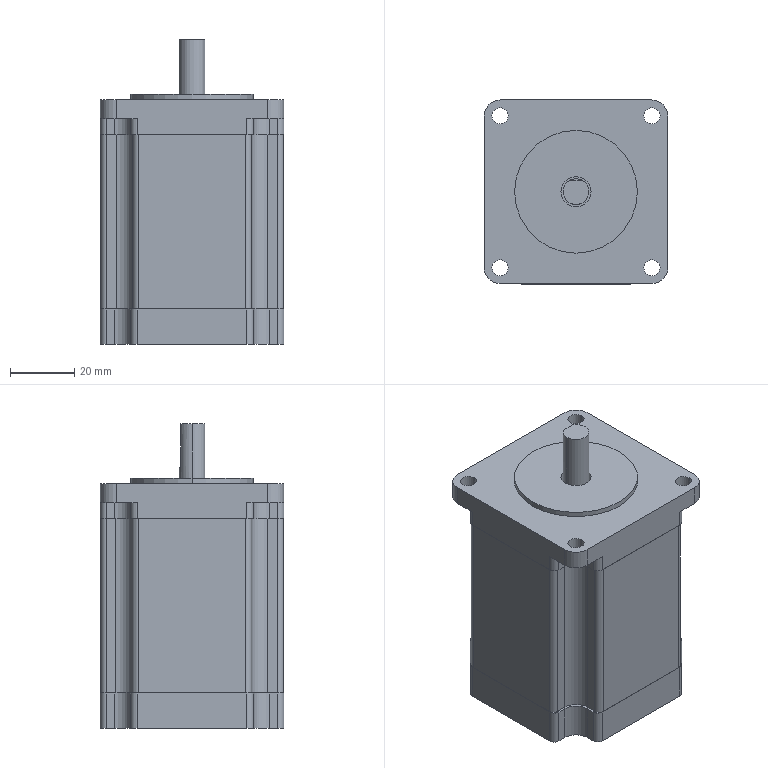Part | 2 solids | 109 faces | box 57 x 57 x 94.6 mm | volume 221170 mm3 | cylinder 56 | plane 51 | cone 2 | commonest cylinder face diameters 4 x16 10 x16 3.8 x8 5 x8 9.35 x4 8 x2